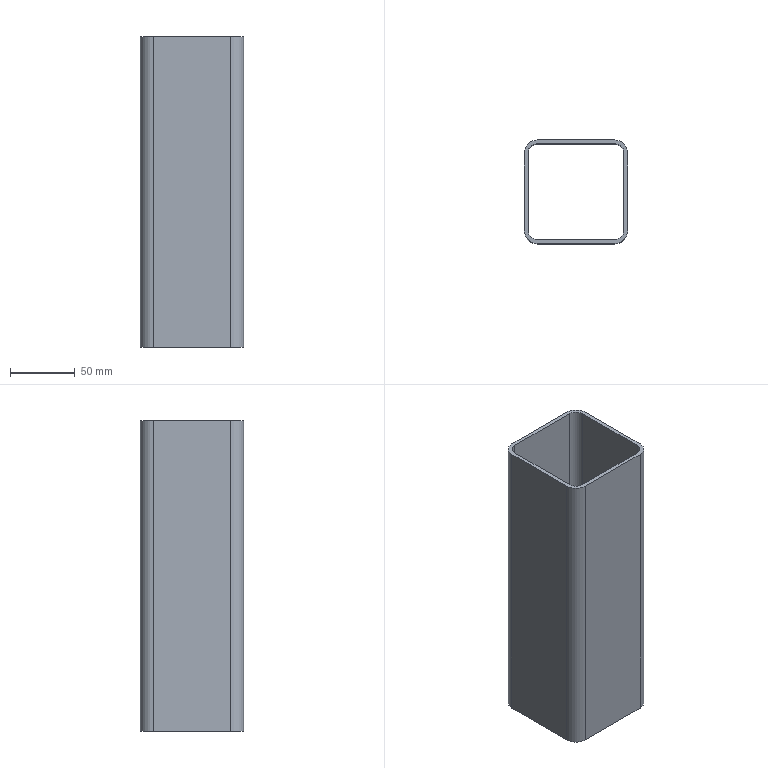Part | STEP file | 1 solid | 18 faces | box 80 x 80 x 240 mm | volume 211253 mm3 | plane 10 | cylinder 8 | commonest cylinder face diameters 14 x4 20 x4
STEP:
#1=CARTESIAN_POINT('',(0.,0.,0.));
#2=DIRECTION('',(0.,0.,1.));
#3=DIRECTION('',(1.,0.,0.));
#4=AXIS2_PLACEMENT_3D('',#1,#2,#3);
#5=CARTESIAN_POINT('',(-30.,40.,120.));
#6=VERTEX_POINT('',#5);
#7=CARTESIAN_POINT('',(-40.,30.,120.));
#8=VERTEX_POINT('',#7);
#9=CARTESIAN_POINT('',(-30.,30.,120.));
#10=DIRECTION('',(0.,0.,1.));
#11=DIRECTION('',(1.,0.,0.));
#12=AXIS2_PLACEMENT_3D('',#9,#10,#11);
#13=CIRCLE('',#12,10.);
#14=CARTESIAN_POINT('',(-30.,30.,120.));
#15=DIRECTION('',(0.,0.,1.));
#16=DIRECTION('',(1.,0.,0.));
#17=AXIS2_PLACEMENT_3D('',#14,#15,#16);
#18=PLANE('',#17);
#19=CARTESIAN_POINT('',(0.,0.));
#20=DIRECTION('',(1.,0.));
#21=AXIS2_PLACEMENT_2D('',#19,#20);
#22=CIRCLE('',#21,10.);
#23=(GEOMETRIC_REPRESENTATION_CONTEXT(2)PARAMETRIC_REPRESENTATION_CONTEXT()REPRESENTATION_CONTEXT('',''));
#24=DEFINITIONAL_REPRESENTATION('',(#22),#23);
#25=PCURVE('',#18,#24);
#26=CARTESIAN_POINT('',(-30.,30.,120.));
#27=DIRECTION('',(0.,0.,-1.));
#28=DIRECTION('',(-1.,0.,0.));
#29=AXIS2_PLACEMENT_3D('',#26,#27,#28);
#30=CYLINDRICAL_SURFACE('',#29,10.);
#31=CARTESIAN_POINT('',(3.142,0.));
#32=DIRECTION('',(-1.,0.));
#33=VECTOR('',#32,1.);
#34=LINE('',#31,#33);
#35=(GEOMETRIC_REPRESENTATION_CONTEXT(2)PARAMETRIC_REPRESENTATION_CONTEXT()REPRESENTATION_CONTEXT('',''));
#36=DEFINITIONAL_REPRESENTATION('',(#34),#35);
#37=PCURVE('',#30,#36);
#38=SURFACE_CURVE('',#13,(#25,#37),.PCURVE_S1.);
#39=EDGE_CURVE('',#6,#8,#38,.T.);
#40=ORIENTED_EDGE('',*,*,#39,.T.);
#41=CARTESIAN_POINT('',(-40.,-30.,120.));
#42=VERTEX_POINT('',#41);
#43=CARTESIAN_POINT('',(-40.,30.,120.));
#44=DIRECTION('',(0.,-1.,0.));
#45=VECTOR('',#44,1.);
#46=LINE('',#43,#45);
#47=CARTESIAN_POINT('',(-10.,0.));
#48=DIRECTION('',(0.,-1.));
#49=VECTOR('',#48,1.);
#50=LINE('',#47,#49);
#51=(GEOMETRIC_REPRESENTATION_CONTEXT(2)PARAMETRIC_REPRESENTATION_CONTEXT()REPRESENTATION_CONTEXT('',''));
#52=DEFINITIONAL_REPRESENTATION('',(#50),#51);
#53=PCURVE('',#18,#52);
#54=CARTESIAN_POINT('',(-40.,30.,120.));
#55=DIRECTION('',(1.,0.,0.));
#56=DIRECTION('',(0.,1.,0.));
#57=AXIS2_PLACEMENT_3D('',#54,#55,#56);
#58=PLANE('',#57);
#59=CARTESIAN_POINT('',(0.,0.));
#60=DIRECTION('',(-1.,0.));
#61=VECTOR('',#60,1.);
#62=LINE('',#59,#61);
#63=(GEOMETRIC_REPRESENTATION_CONTEXT(2)PARAMETRIC_REPRESENTATION_CONTEXT()REPRESENTATION_CONTEXT('',''));
#64=DEFINITIONAL_REPRESENTATION('',(#62),#63);
#65=PCURVE('',#58,#64);
#66=SURFACE_CURVE('',#46,(#53,#65),.PCURVE_S1.);
#67=EDGE_CURVE('',#8,#42,#66,.T.);
#68=ORIENTED_EDGE('',*,*,#67,.T.);
#69=CARTESIAN_POINT('',(-30.,-40.,120.));
#70=VERTEX_POINT('',#69);
#71=CARTESIAN_POINT('',(-30.,-30.,120.));
#72=DIRECTION('',(0.,0.,1.));
#73=DIRECTION('',(-1.,0.,0.));
#74=AXIS2_PLACEMENT_3D('',#71,#72,#73);
#75=CIRCLE('',#74,10.);
#76=CARTESIAN_POINT('',(0.,-60.));
#77=DIRECTION('',(-1.,0.));
#78=AXIS2_PLACEMENT_2D('',#76,#77);
#79=CIRCLE('',#78,10.);
#80=(GEOMETRIC_REPRESENTATION_CONTEXT(2)PARAMETRIC_REPRESENTATION_CONTEXT()REPRESENTATION_CONTEXT('',''));
#81=DEFINITIONAL_REPRESENTATION('',(#79),#80);
#82=PCURVE('',#18,#81);
#83=CARTESIAN_POINT('',(-30.,-30.,120.));
#84=DIRECTION('',(0.,0.,-1.));
#85=DIRECTION('',(-1.,0.,0.));
#86=AXIS2_PLACEMENT_3D('',#83,#84,#85);
#87=CYLINDRICAL_SURFACE('',#86,10.);
#88=CARTESIAN_POINT('',(6.283,0.));
#89=DIRECTION('',(-1.,0.));
#90=VECTOR('',#89,1.);
#91=LINE('',#88,#90);
#92=(GEOMETRIC_REPRESENTATION_CONTEXT(2)PARAMETRIC_REPRESENTATION_CONTEXT()REPRESENTATION_CONTEXT('',''));
#93=DEFINITIONAL_REPRESENTATION('',(#91),#92);
#94=PCURVE('',#87,#93);
#95=SURFACE_CURVE('',#75,(#82,#94),.PCURVE_S1.);
#96=EDGE_CURVE('',#42,#70,#95,.T.);
#97=ORIENTED_EDGE('',*,*,#96,.T.);
#98=CARTESIAN_POINT('',(30.,-40.,120.));
#99=VERTEX_POINT('',#98);
#100=CARTESIAN_POINT('',(30.,-40.,120.));
#101=DIRECTION('',(1.,0.,0.));
#102=VECTOR('',#101,1.);
#103=LINE('',#100,#102);
#104=CARTESIAN_POINT('',(60.,-70.));
#105=DIRECTION('',(1.,0.));
#106=VECTOR('',#105,1.);
#107=LINE('',#104,#106);
#108=(GEOMETRIC_REPRESENTATION_CONTEXT(2)PARAMETRIC_REPRESENTATION_CONTEXT()REPRESENTATION_CONTEXT('',''));
#109=DEFINITIONAL_REPRESENTATION('',(#107),#108);
#110=PCURVE('',#18,#109);
#111=CARTESIAN_POINT('',(30.,-40.,120.));
#112=DIRECTION('',(0.,1.,0.));
#113=DIRECTION('',(-1.,0.,0.));
#114=AXIS2_PLACEMENT_3D('',#111,#112,#113);
#115=PLANE('',#114);
#116=CARTESIAN_POINT('',(0.,0.));
#117=DIRECTION('',(-1.,0.));
#118=VECTOR('',#117,1.);
#119=LINE('',#116,#118);
#120=(GEOMETRIC_REPRESENTATION_CONTEXT(2)PARAMETRIC_REPRESENTATION_CONTEXT()REPRESENTATION_CONTEXT('',''));
#121=DEFINITIONAL_REPRESENTATION('',(#119),#120);
#122=PCURVE('',#115,#121);
#123=SURFACE_CURVE('',#103,(#110,#122),.PCURVE_S1.);
#124=EDGE_CURVE('',#70,#99,#123,.T.);
#125=ORIENTED_EDGE('',*,*,#124,.T.);
#126=CARTESIAN_POINT('',(40.,-30.,120.));
#127=VERTEX_POINT('',#126);
#128=CARTESIAN_POINT('',(30.,-30.,120.));
#129=DIRECTION('',(0.,0.,1.));
#130=DIRECTION('',(-1.,0.,0.));
#131=AXIS2_PLACEMENT_3D('',#128,#129,#130);
#132=CIRCLE('',#131,10.);
#133=CARTESIAN_POINT('',(60.,-60.));
#134=DIRECTION('',(-1.,0.));
#135=AXIS2_PLACEMENT_2D('',#133,#134);
#136=CIRCLE('',#135,10.);
#137=(GEOMETRIC_REPRESENTATION_CONTEXT(2)PARAMETRIC_REPRESENTATION_CONTEXT()REPRESENTATION_CONTEXT('',''));
#138=DEFINITIONAL_REPRESENTATION('',(#136),#137);
#139=PCURVE('',#18,#138);
#140=CARTESIAN_POINT('',(30.,-30.,120.));
#141=DIRECTION('',(0.,0.,-1.));
#142=DIRECTION('',(-1.,0.,0.));
#143=AXIS2_PLACEMENT_3D('',#140,#141,#142);
#144=CYLINDRICAL_SURFACE('',#143,10.);
#145=CARTESIAN_POINT('',(6.283,0.));
#146=DIRECTION('',(-1.,0.));
#147=VECTOR('',#146,1.);
#148=LINE('',#145,#147);
#149=(GEOMETRIC_REPRESENTATION_CONTEXT(2)PARAMETRIC_REPRESENTATION_CONTEXT()REPRESENTATION_CONTEXT('',''));
#150=DEFINITIONAL_REPRESENTATION('',(#148),#149);
#151=PCURVE('',#144,#150);
#152=SURFACE_CURVE('',#132,(#139,#151),.PCURVE_S1.);
#153=EDGE_CURVE('',#99,#127,#152,.T.);
#154=ORIENTED_EDGE('',*,*,#153,.T.);
#155=CARTESIAN_POINT('',(40.,30.,120.));
#156=VERTEX_POINT('',#155);
#157=CARTESIAN_POINT('',(40.,30.,120.));
#158=DIRECTION('',(0.,1.,0.));
#159=VECTOR('',#158,1.);
#160=LINE('',#157,#159);
#161=CARTESIAN_POINT('',(70.,0.));
#162=DIRECTION('',(0.,1.));
#163=VECTOR('',#162,1.);
#164=LINE('',#161,#163);
#165=(GEOMETRIC_REPRESENTATION_CONTEXT(2)PARAMETRIC_REPRESENTATION_CONTEXT()REPRESENTATION_CONTEXT('',''));
#166=DEFINITIONAL_REPRESENTATION('',(#164),#165);
#167=PCURVE('',#18,#166);
#168=CARTESIAN_POINT('',(40.,30.,120.));
#169=DIRECTION('',(-1.,0.,0.));
#170=DIRECTION('',(0.,-1.,0.));
#171=AXIS2_PLACEMENT_3D('',#168,#169,#170);
#172=PLANE('',#171);
#173=CARTESIAN_POINT('',(0.,0.));
#174=DIRECTION('',(-1.,0.));
#175=VECTOR('',#174,1.);
#176=LINE('',#173,#175);
#177=(GEOMETRIC_REPRESENTATION_CONTEXT(2)PARAMETRIC_REPRESENTATION_CONTEXT()REPRESENTATION_CONTEXT('',''));
#178=DEFINITIONAL_REPRESENTATION('',(#176),#177);
#179=PCURVE('',#172,#178);
#180=SURFACE_CURVE('',#160,(#167,#179),.PCURVE_S1.);
#181=EDGE_CURVE('',#127,#156,#180,.T.);
#182=ORIENTED_EDGE('',*,*,#181,.T.);
#183=CARTESIAN_POINT('',(30.,40.,120.));
#184=VERTEX_POINT('',#183);
#185=CARTESIAN_POINT('',(30.,30.,120.));
#186=DIRECTION('',(0.,0.,1.));
#187=DIRECTION('',(-1.,0.,0.));
#188=AXIS2_PLACEMENT_3D('',#185,#186,#187);
#189=CIRCLE('',#188,10.);
#190=CARTESIAN_POINT('',(60.,0.));
#191=DIRECTION('',(-1.,0.));
#192=AXIS2_PLACEMENT_2D('',#190,#191);
#193=CIRCLE('',#192,10.);
#194=(GEOMETRIC_REPRESENTATION_CONTEXT(2)PARAMETRIC_REPRESENTATION_CONTEXT()REPRESENTATION_CONTEXT('',''));
#195=DEFINITIONAL_REPRESENTATION('',(#193),#194);
#196=PCURVE('',#18,#195);
#197=CARTESIAN_POINT('',(30.,30.,120.));
#198=DIRECTION('',(0.,0.,-1.));
#199=DIRECTION('',(-1.,0.,0.));
#200=AXIS2_PLACEMENT_3D('',#197,#198,#199);
#201=CYLINDRICAL_SURFACE('',#200,10.);
#202=CARTESIAN_POINT('',(6.283,0.));
#203=DIRECTION('',(-1.,0.));
#204=VECTOR('',#203,1.);
#205=LINE('',#202,#204);
#206=(GEOMETRIC_REPRESENTATION_CONTEXT(2)PARAMETRIC_REPRESENTATION_CONTEXT()REPRESENTATION_CONTEXT('',''));
#207=DEFINITIONAL_REPRESENTATION('',(#205),#206);
#208=PCURVE('',#201,#207);
#209=SURFACE_CURVE('',#189,(#196,#208),.PCURVE_S1.);
#210=EDGE_CURVE('',#156,#184,#209,.T.);
#211=ORIENTED_EDGE('',*,*,#210,.T.);
#212=CARTESIAN_POINT('',(30.,40.,120.));
#213=DIRECTION('',(-1.,0.,0.));
#214=VECTOR('',#213,1.);
#215=LINE('',#212,#214);
#216=CARTESIAN_POINT('',(60.,10.));
#217=DIRECTION('',(-1.,0.));
#218=VECTOR('',#217,1.);
#219=LINE('',#216,#218);
#220=(GEOMETRIC_REPRESENTATION_CONTEXT(2)PARAMETRIC_REPRESENTATION_CONTEXT()REPRESENTATION_CONTEXT('',''));
#221=DEFINITIONAL_REPRESENTATION('',(#219),#220);
#222=PCURVE('',#18,#221);
#223=CARTESIAN_POINT('',(30.,40.,120.));
#224=DIRECTION('',(0.,-1.,0.));
#225=DIRECTION('',(1.,0.,0.));
#226=AXIS2_PLACEMENT_3D('',#223,#224,#225);
#227=PLANE('',#226);
#228=CARTESIAN_POINT('',(0.,0.));
#229=DIRECTION('',(-1.,0.));
#230=VECTOR('',#229,1.);
#231=LINE('',#228,#230);
#232=(GEOMETRIC_REPRESENTATION_CONTEXT(2)PARAMETRIC_REPRESENTATION_CONTEXT()REPRESENTATION_CONTEXT('',''));
#233=DEFINITIONAL_REPRESENTATION('',(#231),#232);
#234=PCURVE('',#227,#233);
#235=SURFACE_CURVE('',#215,(#222,#234),.PCURVE_S1.);
#236=EDGE_CURVE('',#184,#6,#235,.T.);
#237=ORIENTED_EDGE('',*,*,#236,.T.);
#238=EDGE_LOOP('',(#40,#68,#97,#125,#154,#182,#211,#237));
#239=FACE_BOUND('',#238,.T.);
#240=CARTESIAN_POINT('',(30.,37.,120.));
#241=VERTEX_POINT('',#240);
#242=CARTESIAN_POINT('',(-30.,37.,120.));
#243=VERTEX_POINT('',#242);
#244=CARTESIAN_POINT('',(30.,37.,120.));
#245=DIRECTION('',(-1.,0.,0.));
#246=VECTOR('',#245,1.);
#247=LINE('',#244,#246);
#248=CARTESIAN_POINT('',(60.,7.));
#249=DIRECTION('',(-1.,0.));
#250=VECTOR('',#249,1.);
#251=LINE('',#248,#250);
#252=(GEOMETRIC_REPRESENTATION_CONTEXT(2)PARAMETRIC_REPRESENTATION_CONTEXT()REPRESENTATION_CONTEXT('',''));
#253=DEFINITIONAL_REPRESENTATION('',(#251),#252);
#254=PCURVE('',#18,#253);
#255=CARTESIAN_POINT('',(30.,37.,120.));
#256=DIRECTION('',(0.,-1.,0.));
#257=DIRECTION('',(0.,0.,-1.));
#258=AXIS2_PLACEMENT_3D('',#255,#256,#257);
#259=PLANE('',#258);
#260=CARTESIAN_POINT('',(0.,0.));
#261=DIRECTION('',(0.,-1.));
#262=VECTOR('',#261,1.);
#263=LINE('',#260,#262);
#264=(GEOMETRIC_REPRESENTATION_CONTEXT(2)PARAMETRIC_REPRESENTATION_CONTEXT()REPRESENTATION_CONTEXT('',''));
#265=DEFINITIONAL_REPRESENTATION('',(#263),#264);
#266=PCURVE('',#259,#265);
#267=SURFACE_CURVE('',#247,(#254,#266),.PCURVE_S1.);
#268=EDGE_CURVE('',#241,#243,#267,.T.);
#269=ORIENTED_EDGE('',*,*,#268,.F.);
#270=CARTESIAN_POINT('',(37.,30.,120.));
#271=VERTEX_POINT('',#270);
#272=CARTESIAN_POINT('',(30.,30.,120.));
#273=DIRECTION('',(0.,0.,1.));
#274=DIRECTION('',(-1.,0.,0.));
#275=AXIS2_PLACEMENT_3D('',#272,#273,#274);
#276=CIRCLE('',#275,7.);
#277=CARTESIAN_POINT('',(60.,0.));
#278=DIRECTION('',(-1.,0.));
#279=AXIS2_PLACEMENT_2D('',#277,#278);
#280=CIRCLE('',#279,7.);
#281=(GEOMETRIC_REPRESENTATION_CONTEXT(2)PARAMETRIC_REPRESENTATION_CONTEXT()REPRESENTATION_CONTEXT('',''));
#282=DEFINITIONAL_REPRESENTATION('',(#280),#281);
#283=PCURVE('',#18,#282);
#284=CARTESIAN_POINT('',(30.,30.,120.));
#285=DIRECTION('',(0.,0.,-1.));
#286=DIRECTION('',(-1.,0.,0.));
#287=AXIS2_PLACEMENT_3D('',#284,#285,#286);
#288=CYLINDRICAL_SURFACE('',#287,7.);
#289=CARTESIAN_POINT('',(6.283,0.));
#290=DIRECTION('',(-1.,0.));
#291=VECTOR('',#290,1.);
#292=LINE('',#289,#291);
#293=(GEOMETRIC_REPRESENTATION_CONTEXT(2)PARAMETRIC_REPRESENTATION_CONTEXT()REPRESENTATION_CONTEXT('',''));
#294=DEFINITIONAL_REPRESENTATION('',(#292),#293);
#295=PCURVE('',#288,#294);
#296=SURFACE_CURVE('',#276,(#283,#295),.PCURVE_S1.);
#297=EDGE_CURVE('',#271,#241,#296,.T.);
#298=ORIENTED_EDGE('',*,*,#297,.F.);
#299=CARTESIAN_POINT('',(37.,-30.,120.));
#300=VERTEX_POINT('',#299);
#301=CARTESIAN_POINT('',(37.,30.,120.));
#302=DIRECTION('',(0.,1.,0.));
#303=VECTOR('',#302,1.);
#304=LINE('',#301,#303);
#305=CARTESIAN_POINT('',(67.,0.));
#306=DIRECTION('',(0.,1.));
#307=VECTOR('',#306,1.);
#308=LINE('',#305,#307);
#309=(GEOMETRIC_REPRESENTATION_CONTEXT(2)PARAMETRIC_REPRESENTATION_CONTEXT()REPRESENTATION_CONTEXT('',''));
#310=DEFINITIONAL_REPRESENTATION('',(#308),#309);
#311=PCURVE('',#18,#310);
#312=CARTESIAN_POINT('',(37.,30.,120.));
#313=DIRECTION('',(-1.,0.,0.));
#314=DIRECTION('',(0.,-1.,0.));
#315=AXIS2_PLACEMENT_3D('',#312,#313,#314);
#316=PLANE('',#315);
#317=CARTESIAN_POINT('',(0.,0.));
#318=DIRECTION('',(-1.,0.));
#319=VECTOR('',#318,1.);
#320=LINE('',#317,#319);
#321=(GEOMETRIC_REPRESENTATION_CONTEXT(2)PARAMETRIC_REPRESENTATION_CONTEXT()REPRESENTATION_CONTEXT('',''));
#322=DEFINITIONAL_REPRESENTATION('',(#320),#321);
#323=PCURVE('',#316,#322);
#324=SURFACE_CURVE('',#304,(#311,#323),.PCURVE_S1.);
#325=EDGE_CURVE('',#300,#271,#324,.T.);
#326=ORIENTED_EDGE('',*,*,#325,.F.);
#327=CARTESIAN_POINT('',(30.,-37.,120.));
#328=VERTEX_POINT('',#327);
#329=CARTESIAN_POINT('',(30.,-30.,120.));
#330=DIRECTION('',(0.,0.,1.));
#331=DIRECTION('',(-1.,0.,0.));
#332=AXIS2_PLACEMENT_3D('',#329,#330,#331);
#333=CIRCLE('',#332,7.);
#334=CARTESIAN_POINT('',(60.,-60.));
#335=DIRECTION('',(-1.,0.));
#336=AXIS2_PLACEMENT_2D('',#334,#335);
#337=CIRCLE('',#336,7.);
#338=(GEOMETRIC_REPRESENTATION_CONTEXT(2)PARAMETRIC_REPRESENTATION_CONTEXT()REPRESENTATION_CONTEXT('',''));
#339=DEFINITIONAL_REPRESENTATION('',(#337),#338);
#340=PCURVE('',#18,#339);
#341=CARTESIAN_POINT('',(30.,-30.,120.));
#342=DIRECTION('',(0.,0.,-1.));
#343=DIRECTION('',(-1.,0.,0.));
#344=AXIS2_PLACEMENT_3D('',#341,#342,#343);
#345=CYLINDRICAL_SURFACE('',#344,7.);
#346=CARTESIAN_POINT('',(6.283,0.));
#347=DIRECTION('',(-1.,0.));
#348=VECTOR('',#347,1.);
#349=LINE('',#346,#348);
#350=(GEOMETRIC_REPRESENTATION_CONTEXT(2)PARAMETRIC_REPRESENTATION_CONTEXT()REPRESENTATION_CONTEXT('',''));
#351=DEFINITIONAL_REPRESENTATION('',(#349),#350);
#352=PCURVE('',#345,#351);
#353=SURFACE_CURVE('',#333,(#340,#352),.PCURVE_S1.);
#354=EDGE_CURVE('',#328,#300,#353,.T.);
#355=ORIENTED_EDGE('',*,*,#354,.F.);
#356=CARTESIAN_POINT('',(-30.,-37.,120.));
#357=VERTEX_POINT('',#356);
#358=CARTESIAN_POINT('',(30.,-37.,120.));
#359=DIRECTION('',(1.,0.,0.));
#360=VECTOR('',#359,1.);
#361=LINE('',#358,#360);
#362=CARTESIAN_POINT('',(60.,-67.));
#363=DIRECTION('',(1.,0.));
#364=VECTOR('',#363,1.);
#365=LINE('',#362,#364);
#366=(GEOMETRIC_REPRESENTATION_CONTEXT(2)PARAMETRIC_REPRESENTATION_CONTEXT()REPRESENTATION_CONTEXT('',''));
#367=DEFINITIONAL_REPRESENTATION('',(#365),#366);
#368=PCURVE('',#18,#367);
#369=CARTESIAN_POINT('',(30.,-37.,120.));
#370=DIRECTION('',(0.,1.,0.));
#371=DIRECTION('',(-1.,0.,0.));
#372=AXIS2_PLACEMENT_3D('',#369,#370,#371);
#373=PLANE('',#372);
#374=CARTESIAN_POINT('',(0.,0.));
#375=DIRECTION('',(-1.,0.));
#376=VECTOR('',#375,1.);
#377=LINE('',#374,#376);
#378=(GEOMETRIC_REPRESENTATION_CONTEXT(2)PARAMETRIC_REPRESENTATION_CONTEXT()REPRESENTATION_CONTEXT('',''));
#379=DEFINITIONAL_REPRESENTATION('',(#377),#378);
#380=PCURVE('',#373,#379);
#381=SURFACE_CURVE('',#361,(#368,#380),.PCURVE_S1.);
#382=EDGE_CURVE('',#357,#328,#381,.T.);
#383=ORIENTED_EDGE('',*,*,#382,.F.);
#384=CARTESIAN_POINT('',(-37.,-30.,120.));
#385=VERTEX_POINT('',#384);
#386=CARTESIAN_POINT('',(-30.,-30.,120.));
#387=DIRECTION('',(0.,0.,1.));
#388=DIRECTION('',(-1.,0.,0.));
#389=AXIS2_PLACEMENT_3D('',#386,#387,#388);
#390=CIRCLE('',#389,7.);
#391=CARTESIAN_POINT('',(0.,-60.));
#392=DIRECTION('',(-1.,0.));
#393=AXIS2_PLACEMENT_2D('',#391,#392);
#394=CIRCLE('',#393,7.);
#395=(GEOMETRIC_REPRESENTATION_CONTEXT(2)PARAMETRIC_REPRESENTATION_CONTEXT()REPRESENTATION_CONTEXT('',''));
#396=DEFINITIONAL_REPRESENTATION('',(#394),#395);
#397=PCURVE('',#18,#396);
#398=CARTESIAN_POINT('',(-30.,-30.,120.));
#399=DIRECTION('',(0.,0.,-1.));
#400=DIRECTION('',(-1.,0.,0.));
#401=AXIS2_PLACEMENT_3D('',#398,#399,#400);
#402=CYLINDRICAL_SURFACE('',#401,7.);
#403=CARTESIAN_POINT('',(6.283,0.));
#404=DIRECTION('',(-1.,0.));
#405=VECTOR('',#404,1.);
#406=LINE('',#403,#405);
#407=(GEOMETRIC_REPRESENTATION_CONTEXT(2)PARAMETRIC_REPRESENTATION_CONTEXT()REPRESENTATION_CONTEXT('',''));
#408=DEFINITIONAL_REPRESENTATION('',(#406),#407);
#409=PCURVE('',#402,#408);
#410=SURFACE_CURVE('',#390,(#397,#409),.PCURVE_S1.);
#411=EDGE_CURVE('',#385,#357,#410,.T.);
#412=ORIENTED_EDGE('',*,*,#411,.F.);
#413=CARTESIAN_POINT('',(-37.,30.,120.));
#414=VERTEX_POINT('',#413);
#415=CARTESIAN_POINT('',(-37.,30.,120.));
#416=DIRECTION('',(0.,-1.,0.));
#417=VECTOR('',#416,1.);
#418=LINE('',#415,#417);
#419=CARTESIAN_POINT('',(-7.,0.));
#420=DIRECTION('',(0.,-1.));
#421=VECTOR('',#420,1.);
#422=LINE('',#419,#421);
#423=(GEOMETRIC_REPRESENTATION_CONTEXT(2)PARAMETRIC_REPRESENTATION_CONTEXT()REPRESENTATION_CONTEXT('',''));
#424=DEFINITIONAL_REPRESENTATION('',(#422),#423);
#425=PCURVE('',#18,#424);
#426=CARTESIAN_POINT('',(-37.,30.,120.));
#427=DIRECTION('',(1.,0.,0.));
#428=DIRECTION('',(0.,0.,-1.));
#429=AXIS2_PLACEMENT_3D('',#426,#427,#428);
#430=PLANE('',#429);
#431=CARTESIAN_POINT('',(0.,0.));
#432=DIRECTION('',(0.,-1.));
#433=VECTOR('',#432,1.);
#434=LINE('',#431,#433);
#435=(GEOMETRIC_REPRESENTATION_CONTEXT(2)PARAMETRIC_REPRESENTATION_CONTEXT()REPRESENTATION_CONTEXT('',''));
#436=DEFINITIONAL_REPRESENTATION('',(#434),#435);
#437=PCURVE('',#430,#436);
#438=SURFACE_CURVE('',#418,(#425,#437),.PCURVE_S1.);
#439=EDGE_CURVE('',#414,#385,#438,.T.);
#440=ORIENTED_EDGE('',*,*,#439,.F.);
#441=CARTESIAN_POINT('',(-30.,30.,120.));
#442=DIRECTION('',(0.,0.,1.));
#443=DIRECTION('',(1.,0.,0.));
#444=AXIS2_PLACEMENT_3D('',#441,#442,#443);
#445=CIRCLE('',#444,7.);
#446=CARTESIAN_POINT('',(0.,0.));
#447=DIRECTION('',(1.,0.));
#448=AXIS2_PLACEMENT_2D('',#446,#447);
#449=CIRCLE('',#448,7.);
#450=(GEOMETRIC_REPRESENTATION_CONTEXT(2)PARAMETRIC_REPRESENTATION_CONTEXT()REPRESENTATION_CONTEXT('',''));
#451=DEFINITIONAL_REPRESENTATION('',(#449),#450);
#452=PCURVE('',#18,#451);
#453=CARTESIAN_POINT('',(-30.,30.,120.));
#454=DIRECTION('',(0.,0.,-1.));
#455=DIRECTION('',(-1.,0.,0.));
#456=AXIS2_PLACEMENT_3D('',#453,#454,#455);
#457=CYLINDRICAL_SURFACE('',#456,7.);
#458=CARTESIAN_POINT('',(3.142,0.));
#459=DIRECTION('',(-1.,0.));
#460=VECTOR('',#459,1.);
#461=LINE('',#458,#460);
#462=(GEOMETRIC_REPRESENTATION_CONTEXT(2)PARAMETRIC_REPRESENTATION_CONTEXT()REPRESENTATION_CONTEXT('',''));
#463=DEFINITIONAL_REPRESENTATION('',(#461),#462);
#464=PCURVE('',#457,#463);
#465=SURFACE_CURVE('',#445,(#452,#464),.PCURVE_S1.);
#466=EDGE_CURVE('',#243,#414,#465,.T.);
#467=ORIENTED_EDGE('',*,*,#466,.F.);
#468=EDGE_LOOP('',(#269,#298,#326,#355,#383,#412,#440,#467));
#469=FACE_BOUND('',#468,.T.);
#470=ADVANCED_FACE('',(#239,#469),#18,.T.);
#471=CARTESIAN_POINT('',(-30.,40.,-120.));
#472=VERTEX_POINT('',#471);
#473=CARTESIAN_POINT('',(-40.,30.,-120.));
#474=VERTEX_POINT('',#473);
#475=CARTESIAN_POINT('',(-30.,30.,-120.));
#476=DIRECTION('',(0.,0.,1.));
#477=DIRECTION('',(1.,0.,0.));
#478=AXIS2_PLACEMENT_3D('',#475,#476,#477);
#479=CIRCLE('',#478,10.);
#480=CARTESIAN_POINT('',(-30.,30.,-120.));
#481=DIRECTION('',(0.,0.,1.));
#482=DIRECTION('',(1.,0.,0.));
#483=AXIS2_PLACEMENT_3D('',#480,#481,#482);
#484=PLANE('',#483);
#485=CARTESIAN_POINT('',(0.,0.));
#486=DIRECTION('',(1.,0.));
#487=AXIS2_PLACEMENT_2D('',#485,#486);
#488=CIRCLE('',#487,10.);
#489=(GEOMETRIC_REPRESENTATION_CONTEXT(2)PARAMETRIC_REPRESENTATION_CONTEXT()REPRESENTATION_CONTEXT('',''));
#490=DEFINITIONAL_REPRESENTATION('',(#488),#489);
#491=PCURVE('',#484,#490);
#492=CARTESIAN_POINT('',(3.142,240.));
#493=DIRECTION('',(-1.,0.));
#494=VECTOR('',#493,1.);
#495=LINE('',#492,#494);
#496=(GEOMETRIC_REPRESENTATION_CONTEXT(2)PARAMETRIC_REPRESENTATION_CONTEXT()REPRESENTATION_CONTEXT('',''));
#497=DEFINITIONAL_REPRESENTATION('',(#495),#496);
#498=PCURVE('',#30,#497);
#499=SURFACE_CURVE('',#479,(#491,#498),.PCURVE_S1.);
#500=EDGE_CURVE('',#472,#474,#499,.T.);
#501=ORIENTED_EDGE('',*,*,#500,.F.);
#502=CARTESIAN_POINT('',(30.,40.,-120.));
#503=VERTEX_POINT('',#502);
#504=CARTESIAN_POINT('',(30.,40.,-120.));
#505=DIRECTION('',(-1.,0.,0.));
#506=VECTOR('',#505,1.);
#507=LINE('',#504,#506);
#508=CARTESIAN_POINT('',(60.,10.));
#509=DIRECTION('',(-1.,0.));
#510=VECTOR('',#509,1.);
#511=LINE('',#508,#510);
#512=(GEOMETRIC_REPRESENTATION_CONTEXT(2)PARAMETRIC_REPRESENTATION_CONTEXT()REPRESENTATION_CONTEXT('',''));
#513=DEFINITIONAL_REPRESENTATION('',(#511),#512);
#514=PCURVE('',#484,#513);
#515=CARTESIAN_POINT('',(0.,-240.));
#516=DIRECTION('',(-1.,0.));
#517=VECTOR('',#516,1.);
#518=LINE('',#515,#517);
#519=(GEOMETRIC_REPRESENTATION_CONTEXT(2)PARAMETRIC_REPRESENTATION_CONTEXT()REPRESENTATION_CONTEXT('',''));
#520=DEFINITIONAL_REPRESENTATION('',(#518),#519);
#521=PCURVE('',#227,#520);
#522=SURFACE_CURVE('',#507,(#514,#521),.PCURVE_S1.);
#523=EDGE_CURVE('',#503,#472,#522,.T.);
#524=ORIENTED_EDGE('',*,*,#523,.F.);
#525=CARTESIAN_POINT('',(40.,30.,-120.));
#526=VERTEX_POINT('',#525);
#527=CARTESIAN_POINT('',(30.,30.,-120.));
#528=DIRECTION('',(0.,0.,1.));
#529=DIRECTION('',(-1.,0.,0.));
#530=AXIS2_PLACEMENT_3D('',#527,#528,#529);
#531=CIRCLE('',#530,10.);
#532=CARTESIAN_POINT('',(60.,0.));
#533=DIRECTION('',(-1.,0.));
#534=AXIS2_PLACEMENT_2D('',#532,#533);
#535=CIRCLE('',#534,10.);
#536=(GEOMETRIC_REPRESENTATION_CONTEXT(2)PARAMETRIC_REPRESENTATION_CONTEXT()REPRESENTATION_CONTEXT('',''));
#537=DEFINITIONAL_REPRESENTATION('',(#535),#536);
#538=PCURVE('',#484,#537);
#539=CARTESIAN_POINT('',(6.283,240.));
#540=DIRECTION('',(-1.,0.));
#541=VECTOR('',#540,1.);
#542=LINE('',#539,#541);
#543=(GEOMETRIC_REPRESENTATION_CONTEXT(2)PARAMETRIC_REPRESENTATION_CONTEXT()REPRESENTATION_CONTEXT('',''));
#544=DEFINITIONAL_REPRESENTATION('',(#542),#543);
#545=PCURVE('',#201,#544);
#546=SURFACE_CURVE('',#531,(#538,#545),.PCURVE_S1.);
#547=EDGE_CURVE('',#526,#503,#546,.T.);
#548=ORIENTED_EDGE('',*,*,#547,.F.);
#549=CARTESIAN_POINT('',(40.,-30.,-120.));
#550=VERTEX_POINT('',#549);
#551=CARTESIAN_POINT('',(40.,30.,-120.));
#552=DIRECTION('',(0.,1.,0.));
#553=VECTOR('',#552,1.);
#554=LINE('',#551,#553);
#555=CARTESIAN_POINT('',(70.,0.));
#556=DIRECTION('',(0.,1.));
#557=VECTOR('',#556,1.);
#558=LINE('',#555,#557);
#559=(GEOMETRIC_REPRESENTATION_CONTEXT(2)PARAMETRIC_REPRESENTATION_CONTEXT()REPRESENTATION_CONTEXT('',''));
#560=DEFINITIONAL_REPRESENTATION('',(#558),#559);
#561=PCURVE('',#484,#560);
#562=CARTESIAN_POINT('',(0.,-240.));
#563=DIRECTION('',(-1.,0.));
#564=VECTOR('',#563,1.);
#565=LINE('',#562,#564);
#566=(GEOMETRIC_REPRESENTATION_CONTEXT(2)PARAMETRIC_REPRESENTATION_CONTEXT()REPRESENTATION_CONTEXT('',''));
#567=DEFINITIONAL_REPRESENTATION('',(#565),#566);
#568=PCURVE('',#172,#567);
#569=SURFACE_CURVE('',#554,(#561,#568),.PCURVE_S1.);
#570=EDGE_CURVE('',#550,#526,#569,.T.);
#571=ORIENTED_EDGE('',*,*,#570,.F.);
#572=CARTESIAN_POINT('',(30.,-40.,-120.));
#573=VERTEX_POINT('',#572);
#574=CARTESIAN_POINT('',(30.,-30.,-120.));
#575=DIRECTION('',(0.,0.,1.));
#576=DIRECTION('',(-1.,0.,0.));
#577=AXIS2_PLACEMENT_3D('',#574,#575,#576);
#578=CIRCLE('',#577,10.);
#579=CARTESIAN_POINT('',(60.,-60.));
#580=DIRECTION('',(-1.,0.));
#581=AXIS2_PLACEMENT_2D('',#579,#580);
#582=CIRCLE('',#581,10.);
#583=(GEOMETRIC_REPRESENTATION_CONTEXT(2)PARAMETRIC_REPRESENTATION_CONTEXT()REPRESENTATION_CONTEXT('',''));
#584=DEFINITIONAL_REPRESENTATION('',(#582),#583);
#585=PCURVE('',#484,#584);
#586=CARTESIAN_POINT('',(6.283,240.));
#587=DIRECTION('',(-1.,0.));
#588=VECTOR('',#587,1.);
#589=LINE('',#586,#588);
#590=(GEOMETRIC_REPRESENTATION_CONTEXT(2)PARAMETRIC_REPRESENTATION_CONTEXT()REPRESENTATION_CONTEXT('',''));
#591=DEFINITIONAL_REPRESENTATION('',(#589),#590);
#592=PCURVE('',#144,#591);
#593=SURFACE_CURVE('',#578,(#585,#592),.PCURVE_S1.);
#594=EDGE_CURVE('',#573,#550,#593,.T.);
#595=ORIENTED_EDGE('',*,*,#594,.F.);
#596=CARTESIAN_POINT('',(-30.,-40.,-120.));
#597=VERTEX_POINT('',#596);
#598=CARTESIAN_POINT('',(30.,-40.,-120.));
#599=DIRECTION('',(1.,0.,0.));
#600=VECTOR('',#599,1.);
#601=LINE('',#598,#600);
#602=CARTESIAN_POINT('',(60.,-70.));
#603=DIRECTION('',(1.,0.));
#604=VECTOR('',#603,1.);
#605=LINE('',#602,#604);
#606=(GEOMETRIC_REPRESENTATION_CONTEXT(2)PARAMETRIC_REPRESENTATION_CONTEXT()REPRESENTATION_CONTEXT('',''));
#607=DEFINITIONAL_REPRESENTATION('',(#605),#606);
#608=PCURVE('',#484,#607);
#609=CARTESIAN_POINT('',(0.,-240.));
#610=DIRECTION('',(-1.,0.));
#611=VECTOR('',#610,1.);
#612=LINE('',#609,#611);
#613=(GEOMETRIC_REPRESENTATION_CONTEXT(2)PARAMETRIC_REPRESENTATION_CONTEXT()REPRESENTATION_CONTEXT('',''));
#614=DEFINITIONAL_REPRESENTATION('',(#612),#613);
#615=PCURVE('',#115,#614);
#616=SURFACE_CURVE('',#601,(#608,#615),.PCURVE_S1.);
#617=EDGE_CURVE('',#597,#573,#616,.T.);
#618=ORIENTED_EDGE('',*,*,#617,.F.);
#619=CARTESIAN_POINT('',(-40.,-30.,-120.));
#620=VERTEX_POINT('',#619);
#621=CARTESIAN_POINT('',(-30.,-30.,-120.));
#622=DIRECTION('',(0.,0.,1.));
#623=DIRECTION('',(-1.,0.,0.));
#624=AXIS2_PLACEMENT_3D('',#621,#622,#623);
#625=CIRCLE('',#624,10.);
#626=CARTESIAN_POINT('',(0.,-60.));
#627=DIRECTION('',(-1.,0.));
#628=AXIS2_PLACEMENT_2D('',#626,#627);
#629=CIRCLE('',#628,10.);
#630=(GEOMETRIC_REPRESENTATION_CONTEXT(2)PARAMETRIC_REPRESENTATION_CONTEXT()REPRESENTATION_CONTEXT('',''));
#631=DEFINITIONAL_REPRESENTATION('',(#629),#630);
#632=PCURVE('',#484,#631);
#633=CARTESIAN_POINT('',(6.283,240.));
#634=DIRECTION('',(-1.,0.));
#635=VECTOR('',#634,1.);
#636=LINE('',#633,#635);
#637=(GEOMETRIC_REPRESENTATION_CONTEXT(2)PARAMETRIC_REPRESENTATION_CONTEXT()REPRESENTATION_CONTEXT('',''));
#638=DEFINITIONAL_REPRESENTATION('',(#636),#637);
#639=PCURVE('',#87,#638);
#640=SURFACE_CURVE('',#625,(#632,#639),.PCURVE_S1.);
#641=EDGE_CURVE('',#620,#597,#640,.T.);
#642=ORIENTED_EDGE('',*,*,#641,.F.);
#643=CARTESIAN_POINT('',(-40.,30.,-120.));
#644=DIRECTION('',(0.,-1.,0.));
#645=VECTOR('',#644,1.);
#646=LINE('',#643,#645);
#647=CARTESIAN_POINT('',(-10.,0.));
#648=DIRECTION('',(0.,-1.));
#649=VECTOR('',#648,1.);
#650=LINE('',#647,#649);
#651=(GEOMETRIC_REPRESENTATION_CONTEXT(2)PARAMETRIC_REPRESENTATION_CONTEXT()REPRESENTATION_CONTEXT('',''));
#652=DEFINITIONAL_REPRESENTATION('',(#650),#651);
#653=PCURVE('',#484,#652);
#654=CARTESIAN_POINT('',(0.,-240.));
#655=DIRECTION('',(-1.,0.));
#656=VECTOR('',#655,1.);
#657=LINE('',#654,#656);
#658=(GEOMETRIC_REPRESENTATION_CONTEXT(2)PARAMETRIC_REPRESENTATION_CONTEXT()REPRESENTATION_CONTEXT('',''));
#659=DEFINITIONAL_REPRESENTATION('',(#657),#658);
#660=PCURVE('',#58,#659);
#661=SURFACE_CURVE('',#646,(#653,#660),.PCURVE_S1.);
#662=EDGE_CURVE('',#474,#620,#661,.T.);
#663=ORIENTED_EDGE('',*,*,#662,.F.);
#664=EDGE_LOOP('',(#501,#524,#548,#571,#595,#618,#642,#663));
#665=FACE_BOUND('',#664,.T.);
#666=CARTESIAN_POINT('',(37.,30.,-120.));
#667=VERTEX_POINT('',#666);
#668=CARTESIAN_POINT('',(30.,37.,-120.));
#669=VERTEX_POINT('',#668);
#670=CARTESIAN_POINT('',(30.,30.,-120.));
#671=DIRECTION('',(0.,0.,1.));
#672=DIRECTION('',(-1.,0.,0.));
#673=AXIS2_PLACEMENT_3D('',#670,#671,#672);
#674=CIRCLE('',#673,7.);
#675=CARTESIAN_POINT('',(60.,0.));
#676=DIRECTION('',(-1.,0.));
#677=AXIS2_PLACEMENT_2D('',#675,#676);
#678=CIRCLE('',#677,7.);
#679=(GEOMETRIC_REPRESENTATION_CONTEXT(2)PARAMETRIC_REPRESENTATION_CONTEXT()REPRESENTATION_CONTEXT('',''));
#680=DEFINITIONAL_REPRESENTATION('',(#678),#679);
#681=PCURVE('',#484,#680);
#682=CARTESIAN_POINT('',(6.283,240.));
#683=DIRECTION('',(-1.,0.));
#684=VECTOR('',#683,1.);
#685=LINE('',#682,#684);
#686=(GEOMETRIC_REPRESENTATION_CONTEXT(2)PARAMETRIC_REPRESENTATION_CONTEXT()REPRESENTATION_CONTEXT('',''));
#687=DEFINITIONAL_REPRESENTATION('',(#685),#686);
#688=PCURVE('',#288,#687);
#689=SURFACE_CURVE('',#674,(#681,#688),.PCURVE_S1.);
#690=EDGE_CURVE('',#667,#669,#689,.T.);
#691=ORIENTED_EDGE('',*,*,#690,.T.);
#692=CARTESIAN_POINT('',(-30.,37.,-120.));
#693=VERTEX_POINT('',#692);
#694=CARTESIAN_POINT('',(30.,37.,-120.));
#695=DIRECTION('',(-1.,0.,0.));
#696=VECTOR('',#695,1.);
#697=LINE('',#694,#696);
#698=CARTESIAN_POINT('',(60.,7.));
#699=DIRECTION('',(-1.,0.));
#700=VECTOR('',#699,1.);
#701=LINE('',#698,#700);
#702=(GEOMETRIC_REPRESENTATION_CONTEXT(2)PARAMETRIC_REPRESENTATION_CONTEXT()REPRESENTATION_CONTEXT('',''));
#703=DEFINITIONAL_REPRESENTATION('',(#701),#702);
#704=PCURVE('',#484,#703);
#705=CARTESIAN_POINT('',(240.,0.));
#706=DIRECTION('',(0.,-1.));
#707=VECTOR('',#706,1.);
#708=LINE('',#705,#707);
#709=(GEOMETRIC_REPRESENTATION_CONTEXT(2)PARAMETRIC_REPRESENTATION_CONTEXT()REPRESENTATION_CONTEXT('',''));
#710=DEFINITIONAL_REPRESENTATION('',(#708),#709);
#711=PCURVE('',#259,#710);
#712=SURFACE_CURVE('',#697,(#704,#711),.PCURVE_S1.);
#713=EDGE_CURVE('',#669,#693,#712,.T.);
#714=ORIENTED_EDGE('',*,*,#713,.T.);
#715=CARTESIAN_POINT('',(-37.,30.,-120.));
#716=VERTEX_POINT('',#715);
#717=CARTESIAN_POINT('',(-30.,30.,-120.));
#718=DIRECTION('',(0.,0.,1.));
#719=DIRECTION('',(1.,0.,0.));
#720=AXIS2_PLACEMENT_3D('',#717,#718,#719);
#721=CIRCLE('',#720,7.);
#722=CARTESIAN_POINT('',(0.,0.));
#723=DIRECTION('',(1.,0.));
#724=AXIS2_PLACEMENT_2D('',#722,#723);
#725=CIRCLE('',#724,7.);
#726=(GEOMETRIC_REPRESENTATION_CONTEXT(2)PARAMETRIC_REPRESENTATION_CONTEXT()REPRESENTATION_CONTEXT('',''));
#727=DEFINITIONAL_REPRESENTATION('',(#725),#726);
#728=PCURVE('',#484,#727);
#729=CARTESIAN_POINT('',(3.142,240.));
#730=DIRECTION('',(-1.,0.));
#731=VECTOR('',#730,1.);
#732=LINE('',#729,#731);
#733=(GEOMETRIC_REPRESENTATION_CONTEXT(2)PARAMETRIC_REPRESENTATION_CONTEXT()REPRESENTATION_CONTEXT('',''));
#734=DEFINITIONAL_REPRESENTATION('',(#732),#733);
#735=PCURVE('',#457,#734);
#736=SURFACE_CURVE('',#721,(#728,#735),.PCURVE_S1.);
#737=EDGE_CURVE('',#693,#716,#736,.T.);
#738=ORIENTED_EDGE('',*,*,#737,.T.);
#739=CARTESIAN_POINT('',(-37.,-30.,-120.));
#740=VERTEX_POINT('',#739);
#741=CARTESIAN_POINT('',(-37.,30.,-120.));
#742=DIRECTION('',(0.,-1.,0.));
#743=VECTOR('',#742,1.);
#744=LINE('',#741,#743);
#745=CARTESIAN_POINT('',(-7.,0.));
#746=DIRECTION('',(0.,-1.));
#747=VECTOR('',#746,1.);
#748=LINE('',#745,#747);
#749=(GEOMETRIC_REPRESENTATION_CONTEXT(2)PARAMETRIC_REPRESENTATION_CONTEXT()REPRESENTATION_CONTEXT('',''));
#750=DEFINITIONAL_REPRESENTATION('',(#748),#749);
#751=PCURVE('',#484,#750);
#752=CARTESIAN_POINT('',(240.,0.));
#753=DIRECTION('',(0.,-1.));
#754=VECTOR('',#753,1.);
#755=LINE('',#752,#754);
#756=(GEOMETRIC_REPRESENTATION_CONTEXT(2)PARAMETRIC_REPRESENTATION_CONTEXT()REPRESENTATION_CONTEXT('',''));
#757=DEFINITIONAL_REPRESENTATION('',(#755),#756);
#758=PCURVE('',#430,#757);
#759=SURFACE_CURVE('',#744,(#751,#758),.PCURVE_S1.);
#760=EDGE_CURVE('',#716,#740,#759,.T.);
#761=ORIENTED_EDGE('',*,*,#760,.T.);
#762=CARTESIAN_POINT('',(-30.,-37.,-120.));
#763=VERTEX_POINT('',#762);
#764=CARTESIAN_POINT('',(-30.,-30.,-120.));
#765=DIRECTION('',(0.,0.,1.));
#766=DIRECTION('',(-1.,0.,0.));
#767=AXIS2_PLACEMENT_3D('',#764,#765,#766);
#768=CIRCLE('',#767,7.);
#769=CARTESIAN_POINT('',(0.,-60.));
#770=DIRECTION('',(-1.,0.));
#771=AXIS2_PLACEMENT_2D('',#769,#770);
#772=CIRCLE('',#771,7.);
#773=(GEOMETRIC_REPRESENTATION_CONTEXT(2)PARAMETRIC_REPRESENTATION_CONTEXT()REPRESENTATION_CONTEXT('',''));
#774=DEFINITIONAL_REPRESENTATION('',(#772),#773);
#775=PCURVE('',#484,#774);
#776=CARTESIAN_POINT('',(6.283,240.));
#777=DIRECTION('',(-1.,0.));
#778=VECTOR('',#777,1.);
#779=LINE('',#776,#778);
#780=(GEOMETRIC_REPRESENTATION_CONTEXT(2)PARAMETRIC_REPRESENTATION_CONTEXT()REPRESENTATION_CONTEXT('',''));
#781=DEFINITIONAL_REPRESENTATION('',(#779),#780);
#782=PCURVE('',#402,#781);
#783=SURFACE_CURVE('',#768,(#775,#782),.PCURVE_S1.);
#784=EDGE_CURVE('',#740,#763,#783,.T.);
#785=ORIENTED_EDGE('',*,*,#784,.T.);
#786=CARTESIAN_POINT('',(30.,-37.,-120.));
#787=VERTEX_POINT('',#786);
#788=CARTESIAN_POINT('',(30.,-37.,-120.));
#789=DIRECTION('',(1.,0.,0.));
#790=VECTOR('',#789,1.);
#791=LINE('',#788,#790);
#792=CARTESIAN_POINT('',(60.,-67.));
#793=DIRECTION('',(1.,0.));
#794=VECTOR('',#793,1.);
#795=LINE('',#792,#794);
#796=(GEOMETRIC_REPRESENTATION_CONTEXT(2)PARAMETRIC_REPRESENTATION_CONTEXT()REPRESENTATION_CONTEXT('',''));
#797=DEFINITIONAL_REPRESENTATION('',(#795),#796);
#798=PCURVE('',#484,#797);
#799=CARTESIAN_POINT('',(0.,-240.));
#800=DIRECTION('',(-1.,0.));
#801=VECTOR('',#800,1.);
#802=LINE('',#799,#801);
#803=(GEOMETRIC_REPRESENTATION_CONTEXT(2)PARAMETRIC_REPRESENTATION_CONTEXT()REPRESENTATION_CONTEXT('',''));
#804=DEFINITIONAL_REPRESENTATION('',(#802),#803);
#805=PCURVE('',#373,#804);
#806=SURFACE_CURVE('',#791,(#798,#805),.PCURVE_S1.);
#807=EDGE_CURVE('',#763,#787,#806,.T.);
#808=ORIENTED_EDGE('',*,*,#807,.T.);
#809=CARTESIAN_POINT('',(37.,-30.,-120.));
#810=VERTEX_POINT('',#809);
#811=CARTESIAN_POINT('',(30.,-30.,-120.));
#812=DIRECTION('',(0.,0.,1.));
#813=DIRECTION('',(-1.,0.,0.));
#814=AXIS2_PLACEMENT_3D('',#811,#812,#813);
#815=CIRCLE('',#814,7.);
#816=CARTESIAN_POINT('',(60.,-60.));
#817=DIRECTION('',(-1.,0.));
#818=AXIS2_PLACEMENT_2D('',#816,#817);
#819=CIRCLE('',#818,7.);
#820=(GEOMETRIC_REPRESENTATION_CONTEXT(2)PARAMETRIC_REPRESENTATION_CONTEXT()REPRESENTATION_CONTEXT('',''));
#821=DEFINITIONAL_REPRESENTATION('',(#819),#820);
#822=PCURVE('',#484,#821);
#823=CARTESIAN_POINT('',(6.283,240.));
#824=DIRECTION('',(-1.,0.));
#825=VECTOR('',#824,1.);
#826=LINE('',#823,#825);
#827=(GEOMETRIC_REPRESENTATION_CONTEXT(2)PARAMETRIC_REPRESENTATION_CONTEXT()REPRESENTATION_CONTEXT('',''));
#828=DEFINITIONAL_REPRESENTATION('',(#826),#827);
#829=PCURVE('',#345,#828);
#830=SURFACE_CURVE('',#815,(#822,#829),.PCURVE_S1.);
#831=EDGE_CURVE('',#787,#810,#830,.T.);
#832=ORIENTED_EDGE('',*,*,#831,.T.);
#833=CARTESIAN_POINT('',(37.,30.,-120.));
#834=DIRECTION('',(0.,1.,0.));
#835=VECTOR('',#834,1.);
#836=LINE('',#833,#835);
#837=CARTESIAN_POINT('',(67.,0.));
#838=DIRECTION('',(0.,1.));
#839=VECTOR('',#838,1.);
#840=LINE('',#837,#839);
#841=(GEOMETRIC_REPRESENTATION_CONTEXT(2)PARAMETRIC_REPRESENTATION_CONTEXT()REPRESENTATION_CONTEXT('',''));
#842=DEFINITIONAL_REPRESENTATION('',(#840),#841);
#843=PCURVE('',#484,#842);
#844=CARTESIAN_POINT('',(0.,-240.));
#845=DIRECTION('',(-1.,0.));
#846=VECTOR('',#845,1.);
#847=LINE('',#844,#846);
#848=(GEOMETRIC_REPRESENTATION_CONTEXT(2)PARAMETRIC_REPRESENTATION_CONTEXT()REPRESENTATION_CONTEXT('',''));
#849=DEFINITIONAL_REPRESENTATION('',(#847),#848);
#850=PCURVE('',#316,#849);
#851=SURFACE_CURVE('',#836,(#843,#850),.PCURVE_S1.);
#852=EDGE_CURVE('',#810,#667,#851,.T.);
#853=ORIENTED_EDGE('',*,*,#852,.T.);
#854=EDGE_LOOP('',(#691,#714,#738,#761,#785,#808,#832,#853));
#855=FACE_BOUND('',#854,.T.);
#856=ADVANCED_FACE('',(#665,#855),#484,.F.);
#857=ORIENTED_EDGE('',*,*,#500,.T.);
#858=CARTESIAN_POINT('',(-40.,30.,120.));
#859=DIRECTION('',(0.,0.,-1.));
#860=VECTOR('',#859,1.);
#861=LINE('',#858,#860);
#862=CARTESIAN_POINT('',(0.,0.));
#863=DIRECTION('',(0.,1.));
#864=VECTOR('',#863,1.);
#865=LINE('',#862,#864);
#866=(GEOMETRIC_REPRESENTATION_CONTEXT(2)PARAMETRIC_REPRESENTATION_CONTEXT()REPRESENTATION_CONTEXT('',''));
#867=DEFINITIONAL_REPRESENTATION('',(#865),#866);
#868=PCURVE('',#30,#867);
#869=CARTESIAN_POINT('',(0.,0.));
#870=DIRECTION('',(0.,-1.));
#871=VECTOR('',#870,1.);
#872=LINE('',#869,#871);
#873=(GEOMETRIC_REPRESENTATION_CONTEXT(2)PARAMETRIC_REPRESENTATION_CONTEXT()REPRESENTATION_CONTEXT('',''));
#874=DEFINITIONAL_REPRESENTATION('',(#872),#873);
#875=PCURVE('',#58,#874);
#876=SURFACE_CURVE('',#861,(#868,#875),.PCURVE_S1.);
#877=EDGE_CURVE('',#8,#474,#876,.T.);
#878=ORIENTED_EDGE('',*,*,#877,.F.);
#879=ORIENTED_EDGE('',*,*,#39,.F.);
#880=CARTESIAN_POINT('',(-30.,40.,120.));
#881=DIRECTION('',(0.,0.,-1.));
#882=VECTOR('',#881,1.);
#883=LINE('',#880,#882);
#884=CARTESIAN_POINT('',(1.571,0.));
#885=DIRECTION('',(0.,1.));
#886=VECTOR('',#885,1.);
#887=LINE('',#884,#886);
#888=(GEOMETRIC_REPRESENTATION_CONTEXT(2)PARAMETRIC_REPRESENTATION_CONTEXT()REPRESENTATION_CONTEXT('',''));
#889=DEFINITIONAL_REPRESENTATION('',(#887),#888);
#890=PCURVE('',#30,#889);
#891=CARTESIAN_POINT('',(-60.,0.));
#892=DIRECTION('',(0.,-1.));
#893=VECTOR('',#892,1.);
#894=LINE('',#891,#893);
#895=(GEOMETRIC_REPRESENTATION_CONTEXT(2)PARAMETRIC_REPRESENTATION_CONTEXT()REPRESENTATION_CONTEXT('',''));
#896=DEFINITIONAL_REPRESENTATION('',(#894),#895);
#897=PCURVE('',#227,#896);
#898=SURFACE_CURVE('',#883,(#890,#897),.PCURVE_S1.);
#899=EDGE_CURVE('',#6,#472,#898,.T.);
#900=ORIENTED_EDGE('',*,*,#899,.T.);
#901=EDGE_LOOP('',(#857,#878,#879,#900));
#902=FACE_BOUND('',#901,.T.);
#903=ADVANCED_FACE('',(#902),#30,.T.);
#904=ORIENTED_EDGE('',*,*,#662,.T.);
#905=CARTESIAN_POINT('',(-40.,-30.,120.));
#906=DIRECTION('',(0.,0.,-1.));
#907=VECTOR('',#906,1.);
#908=LINE('',#905,#907);
#909=CARTESIAN_POINT('',(-60.,0.));
#910=DIRECTION('',(0.,-1.));
#911=VECTOR('',#910,1.);
#912=LINE('',#909,#911);
#913=(GEOMETRIC_REPRESENTATION_CONTEXT(2)PARAMETRIC_REPRESENTATION_CONTEXT()REPRESENTATION_CONTEXT('',''));
#914=DEFINITIONAL_REPRESENTATION('',(#912),#913);
#915=PCURVE('',#58,#914);
#916=CARTESIAN_POINT('',(6.283,0.));
#917=DIRECTION('',(0.,1.));
#918=VECTOR('',#917,1.);
#919=LINE('',#916,#918);
#920=(GEOMETRIC_REPRESENTATION_CONTEXT(2)PARAMETRIC_REPRESENTATION_CONTEXT()REPRESENTATION_CONTEXT('',''));
#921=DEFINITIONAL_REPRESENTATION('',(#919),#920);
#922=PCURVE('',#87,#921);
#923=SURFACE_CURVE('',#908,(#915,#922),.PCURVE_S1.);
#924=EDGE_CURVE('',#42,#620,#923,.T.);
#925=ORIENTED_EDGE('',*,*,#924,.F.);
#926=ORIENTED_EDGE('',*,*,#67,.F.);
#927=ORIENTED_EDGE('',*,*,#877,.T.);
#928=EDGE_LOOP('',(#904,#925,#926,#927));
#929=FACE_BOUND('',#928,.T.);
#930=ADVANCED_FACE('',(#929),#58,.F.);
#931=ORIENTED_EDGE('',*,*,#641,.T.);
#932=CARTESIAN_POINT('',(-30.,-40.,120.));
#933=DIRECTION('',(0.,0.,-1.));
#934=VECTOR('',#933,1.);
#935=LINE('',#932,#934);
#936=CARTESIAN_POINT('',(4.712,0.));
#937=DIRECTION('',(0.,1.));
#938=VECTOR('',#937,1.);
#939=LINE('',#936,#938);
#940=(GEOMETRIC_REPRESENTATION_CONTEXT(2)PARAMETRIC_REPRESENTATION_CONTEXT()REPRESENTATION_CONTEXT('',''));
#941=DEFINITIONAL_REPRESENTATION('',(#939),#940);
#942=PCURVE('',#87,#941);
#943=CARTESIAN_POINT('',(60.,0.));
#944=DIRECTION('',(0.,-1.));
#945=VECTOR('',#944,1.);
#946=LINE('',#943,#945);
#947=(GEOMETRIC_REPRESENTATION_CONTEXT(2)PARAMETRIC_REPRESENTATION_CONTEXT()REPRESENTATION_CONTEXT('',''));
#948=DEFINITIONAL_REPRESENTATION('',(#946),#947);
#949=PCURVE('',#115,#948);
#950=SURFACE_CURVE('',#935,(#942,#949),.PCURVE_S1.);
#951=EDGE_CURVE('',#70,#597,#950,.T.);
#952=ORIENTED_EDGE('',*,*,#951,.F.);
#953=ORIENTED_EDGE('',*,*,#96,.F.);
#954=ORIENTED_EDGE('',*,*,#924,.T.);
#955=EDGE_LOOP('',(#931,#952,#953,#954));
#956=FACE_BOUND('',#955,.T.);
#957=ADVANCED_FACE('',(#956),#87,.T.);
#958=ORIENTED_EDGE('',*,*,#617,.T.);
#959=CARTESIAN_POINT('',(30.,-40.,120.));
#960=DIRECTION('',(0.,0.,-1.));
#961=VECTOR('',#960,1.);
#962=LINE('',#959,#961);
#963=CARTESIAN_POINT('',(0.,0.));
#964=DIRECTION('',(0.,-1.));
#965=VECTOR('',#964,1.);
#966=LINE('',#963,#965);
#967=(GEOMETRIC_REPRESENTATION_CONTEXT(2)PARAMETRIC_REPRESENTATION_CONTEXT()REPRESENTATION_CONTEXT('',''));
#968=DEFINITIONAL_REPRESENTATION('',(#966),#967);
#969=PCURVE('',#115,#968);
#970=CARTESIAN_POINT('',(4.712,0.));
#971=DIRECTION('',(0.,1.));
#972=VECTOR('',#971,1.);
#973=LINE('',#970,#972);
#974=(GEOMETRIC_REPRESENTATION_CONTEXT(2)PARAMETRIC_REPRESENTATION_CONTEXT()REPRESENTATION_CONTEXT('',''));
#975=DEFINITIONAL_REPRESENTATION('',(#973),#974);
#976=PCURVE('',#144,#975);
#977=SURFACE_CURVE('',#962,(#969,#976),.PCURVE_S1.);
#978=EDGE_CURVE('',#99,#573,#977,.T.);
#979=ORIENTED_EDGE('',*,*,#978,.F.);
#980=ORIENTED_EDGE('',*,*,#124,.F.);
#981=ORIENTED_EDGE('',*,*,#951,.T.);
#982=EDGE_LOOP('',(#958,#979,#980,#981));
#983=FACE_BOUND('',#982,.T.);
#984=ADVANCED_FACE('',(#983),#115,.F.);
#985=ORIENTED_EDGE('',*,*,#594,.T.);
#986=CARTESIAN_POINT('',(40.,-30.,120.));
#987=DIRECTION('',(0.,0.,-1.));
#988=VECTOR('',#987,1.);
#989=LINE('',#986,#988);
#990=CARTESIAN_POINT('',(3.142,0.));
#991=DIRECTION('',(0.,1.));
#992=VECTOR('',#991,1.);
#993=LINE('',#990,#992);
#994=(GEOMETRIC_REPRESENTATION_CONTEXT(2)PARAMETRIC_REPRESENTATION_CONTEXT()REPRESENTATION_CONTEXT('',''));
#995=DEFINITIONAL_REPRESENTATION('',(#993),#994);
#996=PCURVE('',#144,#995);
#997=CARTESIAN_POINT('',(60.,0.));
#998=DIRECTION('',(0.,-1.));
#999=VECTOR('',#998,1.);
#1000=LINE('',#997,#999);
#1001=(GEOMETRIC_REPRESENTATION_CONTEXT(2)PARAMETRIC_REPRESENTATION_CONTEXT()REPRESENTATION_CONTEXT('',''));
#1002=DEFINITIONAL_REPRESENTATION('',(#1000),#1001);
#1003=PCURVE('',#172,#1002);
#1004=SURFACE_CURVE('',#989,(#996,#1003),.PCURVE_S1.);
#1005=EDGE_CURVE('',#127,#550,#1004,.T.);
#1006=ORIENTED_EDGE('',*,*,#1005,.F.);
#1007=ORIENTED_EDGE('',*,*,#153,.F.);
#1008=ORIENTED_EDGE('',*,*,#978,.T.);
#1009=EDGE_LOOP('',(#985,#1006,#1007,#1008));
#1010=FACE_BOUND('',#1009,.T.);
#1011=ADVANCED_FACE('',(#1010),#144,.T.);
#1012=ORIENTED_EDGE('',*,*,#570,.T.);
#1013=CARTESIAN_POINT('',(40.,30.,120.));
#1014=DIRECTION('',(0.,0.,-1.));
#1015=VECTOR('',#1014,1.);
#1016=LINE('',#1013,#1015);
#1017=CARTESIAN_POINT('',(0.,0.));
#1018=DIRECTION('',(0.,-1.));
#1019=VECTOR('',#1018,1.);
#1020=LINE('',#1017,#1019);
#1021=(GEOMETRIC_REPRESENTATION_CONTEXT(2)PARAMETRIC_REPRESENTATION_CONTEXT()REPRESENTATION_CONTEXT('',''));
#1022=DEFINITIONAL_REPRESENTATION('',(#1020),#1021);
#1023=PCURVE('',#172,#1022);
#1024=CARTESIAN_POINT('',(3.142,0.));
#1025=DIRECTION('',(0.,1.));
#1026=VECTOR('',#1025,1.);
#1027=LINE('',#1024,#1026);
#1028=(GEOMETRIC_REPRESENTATION_CONTEXT(2)PARAMETRIC_REPRESENTATION_CONTEXT()REPRESENTATION_CONTEXT('',''));
#1029=DEFINITIONAL_REPRESENTATION('',(#1027),#1028);
#1030=PCURVE('',#201,#1029);
#1031=SURFACE_CURVE('',#1016,(#1023,#1030),.PCURVE_S1.);
#1032=EDGE_CURVE('',#156,#526,#1031,.T.);
#1033=ORIENTED_EDGE('',*,*,#1032,.F.);
#1034=ORIENTED_EDGE('',*,*,#181,.F.);
#1035=ORIENTED_EDGE('',*,*,#1005,.T.);
#1036=EDGE_LOOP('',(#1012,#1033,#1034,#1035));
#1037=FACE_BOUND('',#1036,.T.);
#1038=ADVANCED_FACE('',(#1037),#172,.F.);
#1039=ORIENTED_EDGE('',*,*,#547,.T.);
#1040=CARTESIAN_POINT('',(30.,40.,120.));
#1041=DIRECTION('',(0.,0.,-1.));
#1042=VECTOR('',#1041,1.);
#1043=LINE('',#1040,#1042);
#1044=CARTESIAN_POINT('',(1.571,0.));
#1045=DIRECTION('',(0.,1.));
#1046=VECTOR('',#1045,1.);
#1047=LINE('',#1044,#1046);
#1048=(GEOMETRIC_REPRESENTATION_CONTEXT(2)PARAMETRIC_REPRESENTATION_CONTEXT()REPRESENTATION_CONTEXT('',''));
#1049=DEFINITIONAL_REPRESENTATION('',(#1047),#1048);
#1050=PCURVE('',#201,#1049);
#1051=CARTESIAN_POINT('',(0.,0.));
#1052=DIRECTION('',(0.,-1.));
#1053=VECTOR('',#1052,1.);
#1054=LINE('',#1051,#1053);
#1055=(GEOMETRIC_REPRESENTATION_CONTEXT(2)PARAMETRIC_REPRESENTATION_CONTEXT()REPRESENTATION_CONTEXT('',''));
#1056=DEFINITIONAL_REPRESENTATION('',(#1054),#1055);
#1057=PCURVE('',#227,#1056);
#1058=SURFACE_CURVE('',#1043,(#1050,#1057),.PCURVE_S1.);
#1059=EDGE_CURVE('',#184,#503,#1058,.T.);
#1060=ORIENTED_EDGE('',*,*,#1059,.F.);
#1061=ORIENTED_EDGE('',*,*,#210,.F.);
#1062=ORIENTED_EDGE('',*,*,#1032,.T.);
#1063=EDGE_LOOP('',(#1039,#1060,#1061,#1062));
#1064=FACE_BOUND('',#1063,.T.);
#1065=ADVANCED_FACE('',(#1064),#201,.T.);
#1066=ORIENTED_EDGE('',*,*,#523,.T.);
#1067=ORIENTED_EDGE('',*,*,#899,.F.);
#1068=ORIENTED_EDGE('',*,*,#236,.F.);
#1069=ORIENTED_EDGE('',*,*,#1059,.T.);
#1070=EDGE_LOOP('',(#1066,#1067,#1068,#1069));
#1071=FACE_BOUND('',#1070,.T.);
#1072=ADVANCED_FACE('',(#1071),#227,.F.);
#1073=CARTESIAN_POINT('',(30.,37.,120.));
#1074=DIRECTION('',(0.,0.,-1.));
#1075=VECTOR('',#1074,1.);
#1076=LINE('',#1073,#1075);
#1077=CARTESIAN_POINT('',(1.571,0.));
#1078=DIRECTION('',(0.,1.));
#1079=VECTOR('',#1078,1.);
#1080=LINE('',#1077,#1079);
#1081=(GEOMETRIC_REPRESENTATION_CONTEXT(2)PARAMETRIC_REPRESENTATION_CONTEXT()REPRESENTATION_CONTEXT('',''));
#1082=DEFINITIONAL_REPRESENTATION('',(#1080),#1081);
#1083=PCURVE('',#288,#1082);
#1084=CARTESIAN_POINT('',(0.,0.));
#1085=DIRECTION('',(1.,0.));
#1086=VECTOR('',#1085,1.);
#1087=LINE('',#1084,#1086);
#1088=(GEOMETRIC_REPRESENTATION_CONTEXT(2)PARAMETRIC_REPRESENTATION_CONTEXT()REPRESENTATION_CONTEXT('',''));
#1089=DEFINITIONAL_REPRESENTATION('',(#1087),#1088);
#1090=PCURVE('',#259,#1089);
#1091=SURFACE_CURVE('',#1076,(#1083,#1090),.PCURVE_S1.);
#1092=EDGE_CURVE('',#241,#669,#1091,.T.);
#1093=ORIENTED_EDGE('',*,*,#1092,.F.);
#1094=ORIENTED_EDGE('',*,*,#297,.F.);
#1095=CARTESIAN_POINT('',(37.,30.,120.));
#1096=DIRECTION('',(0.,0.,-1.));
#1097=VECTOR('',#1096,1.);
#1098=LINE('',#1095,#1097);
#1099=CARTESIAN_POINT('',(3.142,0.));
#1100=DIRECTION('',(0.,1.));
#1101=VECTOR('',#1100,1.);
#1102=LINE('',#1099,#1101);
#1103=(GEOMETRIC_REPRESENTATION_CONTEXT(2)PARAMETRIC_REPRESENTATION_CONTEXT()REPRESENTATION_CONTEXT('',''));
#1104=DEFINITIONAL_REPRESENTATION('',(#1102),#1103);
#1105=PCURVE('',#288,#1104);
#1106=CARTESIAN_POINT('',(0.,0.));
#1107=DIRECTION('',(0.,-1.));
#1108=VECTOR('',#1107,1.);
#1109=LINE('',#1106,#1108);
#1110=(GEOMETRIC_REPRESENTATION_CONTEXT(2)PARAMETRIC_REPRESENTATION_CONTEXT()REPRESENTATION_CONTEXT('',''));
#1111=DEFINITIONAL_REPRESENTATION('',(#1109),#1110);
#1112=PCURVE('',#316,#1111);
#1113=SURFACE_CURVE('',#1098,(#1105,#1112),.PCURVE_S1.);
#1114=EDGE_CURVE('',#271,#667,#1113,.T.);
#1115=ORIENTED_EDGE('',*,*,#1114,.T.);
#1116=ORIENTED_EDGE('',*,*,#690,.T.);
#1117=EDGE_LOOP('',(#1093,#1094,#1115,#1116));
#1118=FACE_BOUND('',#1117,.F.);
#1119=ADVANCED_FACE('',(#1118),#288,.F.);
#1120=ORIENTED_EDGE('',*,*,#713,.F.);
#1121=ORIENTED_EDGE('',*,*,#1092,.F.);
#1122=ORIENTED_EDGE('',*,*,#268,.T.);
#1123=CARTESIAN_POINT('',(-30.,37.,120.));
#1124=DIRECTION('',(0.,0.,-1.));
#1125=VECTOR('',#1124,1.);
#1126=LINE('',#1123,#1125);
#1127=CARTESIAN_POINT('',(0.,-60.));
#1128=DIRECTION('',(1.,0.));
#1129=VECTOR('',#1128,1.);
#1130=LINE('',#1127,#1129);
#1131=(GEOMETRIC_REPRESENTATION_CONTEXT(2)PARAMETRIC_REPRESENTATION_CONTEXT()REPRESENTATION_CONTEXT('',''));
#1132=DEFINITIONAL_REPRESENTATION('',(#1130),#1131);
#1133=PCURVE('',#259,#1132);
#1134=CARTESIAN_POINT('',(1.571,0.));
#1135=DIRECTION('',(0.,1.));
#1136=VECTOR('',#1135,1.);
#1137=LINE('',#1134,#1136);
#1138=(GEOMETRIC_REPRESENTATION_CONTEXT(2)PARAMETRIC_REPRESENTATION_CONTEXT()REPRESENTATION_CONTEXT('',''));
#1139=DEFINITIONAL_REPRESENTATION('',(#1137),#1138);
#1140=PCURVE('',#457,#1139);
#1141=SURFACE_CURVE('',#1126,(#1133,#1140),.PCURVE_S1.);
#1142=EDGE_CURVE('',#243,#693,#1141,.T.);
#1143=ORIENTED_EDGE('',*,*,#1142,.T.);
#1144=EDGE_LOOP('',(#1120,#1121,#1122,#1143));
#1145=FACE_BOUND('',#1144,.T.);
#1146=ADVANCED_FACE('',(#1145),#259,.T.);
#1147=CARTESIAN_POINT('',(-37.,30.,120.));
#1148=DIRECTION('',(0.,0.,-1.));
#1149=VECTOR('',#1148,1.);
#1150=LINE('',#1147,#1149);
#1151=CARTESIAN_POINT('',(0.,0.));
#1152=DIRECTION('',(0.,1.));
#1153=VECTOR('',#1152,1.);
#1154=LINE('',#1151,#1153);
#1155=(GEOMETRIC_REPRESENTATION_CONTEXT(2)PARAMETRIC_REPRESENTATION_CONTEXT()REPRESENTATION_CONTEXT('',''));
#1156=DEFINITIONAL_REPRESENTATION('',(#1154),#1155);
#1157=PCURVE('',#457,#1156);
#1158=CARTESIAN_POINT('',(0.,0.));
#1159=DIRECTION('',(1.,0.));
#1160=VECTOR('',#1159,1.);
#1161=LINE('',#1158,#1160);
#1162=(GEOMETRIC_REPRESENTATION_CONTEXT(2)PARAMETRIC_REPRESENTATION_CONTEXT()REPRESENTATION_CONTEXT('',''));
#1163=DEFINITIONAL_REPRESENTATION('',(#1161),#1162);
#1164=PCURVE('',#430,#1163);
#1165=SURFACE_CURVE('',#1150,(#1157,#1164),.PCURVE_S1.);
#1166=EDGE_CURVE('',#414,#716,#1165,.T.);
#1167=ORIENTED_EDGE('',*,*,#1166,.F.);
#1168=ORIENTED_EDGE('',*,*,#466,.F.);
#1169=ORIENTED_EDGE('',*,*,#1142,.T.);
#1170=ORIENTED_EDGE('',*,*,#737,.T.);
#1171=EDGE_LOOP('',(#1167,#1168,#1169,#1170));
#1172=FACE_BOUND('',#1171,.F.);
#1173=ADVANCED_FACE('',(#1172),#457,.F.);
#1174=ORIENTED_EDGE('',*,*,#760,.F.);
#1175=ORIENTED_EDGE('',*,*,#1166,.F.);
#1176=ORIENTED_EDGE('',*,*,#439,.T.);
#1177=CARTESIAN_POINT('',(-37.,-30.,120.));
#1178=DIRECTION('',(0.,0.,-1.));
#1179=VECTOR('',#1178,1.);
#1180=LINE('',#1177,#1179);
#1181=CARTESIAN_POINT('',(0.,-60.));
#1182=DIRECTION('',(1.,0.));
#1183=VECTOR('',#1182,1.);
#1184=LINE('',#1181,#1183);
#1185=(GEOMETRIC_REPRESENTATION_CONTEXT(2)PARAMETRIC_REPRESENTATION_CONTEXT()REPRESENTATION_CONTEXT('',''));
#1186=DEFINITIONAL_REPRESENTATION('',(#1184),#1185);
#1187=PCURVE('',#430,#1186);
#1188=CARTESIAN_POINT('',(6.283,0.));
#1189=DIRECTION('',(0.,1.));
#1190=VECTOR('',#1189,1.);
#1191=LINE('',#1188,#1190);
#1192=(GEOMETRIC_REPRESENTATION_CONTEXT(2)PARAMETRIC_REPRESENTATION_CONTEXT()REPRESENTATION_CONTEXT('',''));
#1193=DEFINITIONAL_REPRESENTATION('',(#1191),#1192);
#1194=PCURVE('',#402,#1193);
#1195=SURFACE_CURVE('',#1180,(#1187,#1194),.PCURVE_S1.);
#1196=EDGE_CURVE('',#385,#740,#1195,.T.);
#1197=ORIENTED_EDGE('',*,*,#1196,.T.);
#1198=EDGE_LOOP('',(#1174,#1175,#1176,#1197));
#1199=FACE_BOUND('',#1198,.T.);
#1200=ADVANCED_FACE('',(#1199),#430,.T.);
#1201=CARTESIAN_POINT('',(-30.,-37.,120.));
#1202=DIRECTION('',(0.,0.,-1.));
#1203=VECTOR('',#1202,1.);
#1204=LINE('',#1201,#1203);
#1205=CARTESIAN_POINT('',(4.712,0.));
#1206=DIRECTION('',(0.,1.));
#1207=VECTOR('',#1206,1.);
#1208=LINE('',#1205,#1207);
#1209=(GEOMETRIC_REPRESENTATION_CONTEXT(2)PARAMETRIC_REPRESENTATION_CONTEXT()REPRESENTATION_CONTEXT('',''));
#1210=DEFINITIONAL_REPRESENTATION('',(#1208),#1209);
#1211=PCURVE('',#402,#1210);
#1212=CARTESIAN_POINT('',(60.,0.));
#1213=DIRECTION('',(0.,-1.));
#1214=VECTOR('',#1213,1.);
#1215=LINE('',#1212,#1214);
#1216=(GEOMETRIC_REPRESENTATION_CONTEXT(2)PARAMETRIC_REPRESENTATION_CONTEXT()REPRESENTATION_CONTEXT('',''));
#1217=DEFINITIONAL_REPRESENTATION('',(#1215),#1216);
#1218=PCURVE('',#373,#1217);
#1219=SURFACE_CURVE('',#1204,(#1211,#1218),.PCURVE_S1.);
#1220=EDGE_CURVE('',#357,#763,#1219,.T.);
#1221=ORIENTED_EDGE('',*,*,#1220,.F.);
#1222=ORIENTED_EDGE('',*,*,#411,.F.);
#1223=ORIENTED_EDGE('',*,*,#1196,.T.);
#1224=ORIENTED_EDGE('',*,*,#784,.T.);
#1225=EDGE_LOOP('',(#1221,#1222,#1223,#1224));
#1226=FACE_BOUND('',#1225,.F.);
#1227=ADVANCED_FACE('',(#1226),#402,.F.);
#1228=ORIENTED_EDGE('',*,*,#807,.F.);
#1229=ORIENTED_EDGE('',*,*,#1220,.F.);
#1230=ORIENTED_EDGE('',*,*,#382,.T.);
#1231=CARTESIAN_POINT('',(30.,-37.,120.));
#1232=DIRECTION('',(0.,0.,-1.));
#1233=VECTOR('',#1232,1.);
#1234=LINE('',#1231,#1233);
#1235=CARTESIAN_POINT('',(0.,0.));
#1236=DIRECTION('',(0.,-1.));
#1237=VECTOR('',#1236,1.);
#1238=LINE('',#1235,#1237);
#1239=(GEOMETRIC_REPRESENTATION_CONTEXT(2)PARAMETRIC_REPRESENTATION_CONTEXT()REPRESENTATION_CONTEXT('',''));
#1240=DEFINITIONAL_REPRESENTATION('',(#1238),#1239);
#1241=PCURVE('',#373,#1240);
#1242=CARTESIAN_POINT('',(4.712,0.));
#1243=DIRECTION('',(0.,1.));
#1244=VECTOR('',#1243,1.);
#1245=LINE('',#1242,#1244);
#1246=(GEOMETRIC_REPRESENTATION_CONTEXT(2)PARAMETRIC_REPRESENTATION_CONTEXT()REPRESENTATION_CONTEXT('',''));
#1247=DEFINITIONAL_REPRESENTATION('',(#1245),#1246);
#1248=PCURVE('',#345,#1247);
#1249=SURFACE_CURVE('',#1234,(#1241,#1248),.PCURVE_S1.);
#1250=EDGE_CURVE('',#328,#787,#1249,.T.);
#1251=ORIENTED_EDGE('',*,*,#1250,.T.);
#1252=EDGE_LOOP('',(#1228,#1229,#1230,#1251));
#1253=FACE_BOUND('',#1252,.T.);
#1254=ADVANCED_FACE('',(#1253),#373,.T.);
#1255=CARTESIAN_POINT('',(37.,-30.,120.));
#1256=DIRECTION('',(0.,0.,-1.));
#1257=VECTOR('',#1256,1.);
#1258=LINE('',#1255,#1257);
#1259=CARTESIAN_POINT('',(3.142,0.));
#1260=DIRECTION('',(0.,1.));
#1261=VECTOR('',#1260,1.);
#1262=LINE('',#1259,#1261);
#1263=(GEOMETRIC_REPRESENTATION_CONTEXT(2)PARAMETRIC_REPRESENTATION_CONTEXT()REPRESENTATION_CONTEXT('',''));
#1264=DEFINITIONAL_REPRESENTATION('',(#1262),#1263);
#1265=PCURVE('',#345,#1264);
#1266=CARTESIAN_POINT('',(60.,0.));
#1267=DIRECTION('',(0.,-1.));
#1268=VECTOR('',#1267,1.);
#1269=LINE('',#1266,#1268);
#1270=(GEOMETRIC_REPRESENTATION_CONTEXT(2)PARAMETRIC_REPRESENTATION_CONTEXT()REPRESENTATION_CONTEXT('',''));
#1271=DEFINITIONAL_REPRESENTATION('',(#1269),#1270);
#1272=PCURVE('',#316,#1271);
#1273=SURFACE_CURVE('',#1258,(#1265,#1272),.PCURVE_S1.);
#1274=EDGE_CURVE('',#300,#810,#1273,.T.);
#1275=ORIENTED_EDGE('',*,*,#1274,.F.);
#1276=ORIENTED_EDGE('',*,*,#354,.F.);
#1277=ORIENTED_EDGE('',*,*,#1250,.T.);
#1278=ORIENTED_EDGE('',*,*,#831,.T.);
#1279=EDGE_LOOP('',(#1275,#1276,#1277,#1278));
#1280=FACE_BOUND('',#1279,.F.);
#1281=ADVANCED_FACE('',(#1280),#345,.F.);
#1282=ORIENTED_EDGE('',*,*,#852,.F.);
#1283=ORIENTED_EDGE('',*,*,#1274,.F.);
#1284=ORIENTED_EDGE('',*,*,#325,.T.);
#1285=ORIENTED_EDGE('',*,*,#1114,.T.);
#1286=EDGE_LOOP('',(#1282,#1283,#1284,#1285));
#1287=FACE_BOUND('',#1286,.T.);
#1288=ADVANCED_FACE('',(#1287),#316,.T.);
#1289=CLOSED_SHELL('',(#470,#856,#903,#930,#957,#984,#1011,#1038,#1065,#1072,#1119,#1146,#1173,#1200,#1227,#1254,#1281,#1288));
#1290=MANIFOLD_SOLID_BREP('',#1289);
#1291=(LENGTH_UNIT()NAMED_UNIT(*)SI_UNIT(.MILLI.,.METRE.));
#1292=UNCERTAINTY_MEASURE_WITH_UNIT(LENGTH_MEASURE(0.0000001),#1291,'','');
#1293=(NAMED_UNIT(*)PLANE_ANGLE_UNIT()SI_UNIT($,.RADIAN.));
#1294=(NAMED_UNIT(*)SI_UNIT($,.STERADIAN.)SOLID_ANGLE_UNIT());
#1295=(GEOMETRIC_REPRESENTATION_CONTEXT(3)GLOBAL_UNCERTAINTY_ASSIGNED_CONTEXT((#1292))GLOBAL_UNIT_ASSIGNED_CONTEXT((#1291,#1293,#1294))REPRESENTATION_CONTEXT('',''));
#1296=ADVANCED_BREP_SHAPE_REPRESENTATION('',(#4,#1290),#1295);